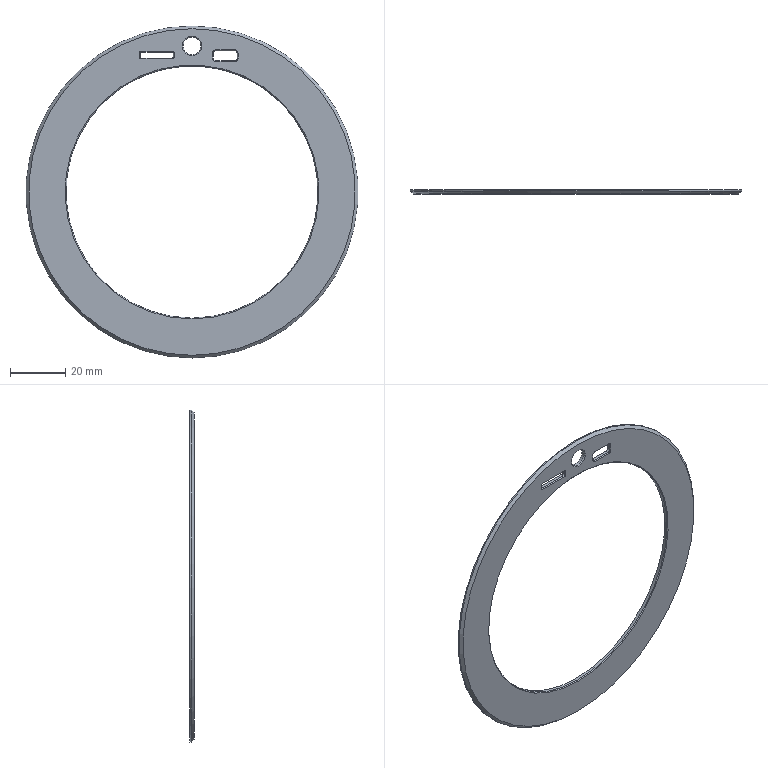Part | NX | 1 solid | 40 faces | box 119.8 x 1.45 x 119.8 mm | volume 6583 mm3 | plane 18 | cylinder 11 | cone 11 | commonest cylinder face diameters 0.6 x4 2 x4 6.4 x1 91 x1 119.8 x1
STEP:
#1=CARTESIAN_POINT('',(-7.04,-1.45,48.03));
#2=VERTEX_POINT('',#1);
#3=CARTESIAN_POINT('',(-18.44,-1.45,48.03));
#4=VERTEX_POINT('',#3);
#5=CARTESIAN_POINT('',(0.,-1.45,48.03));
#6=DIRECTION('',(-1.,0.,0.));
#7=VECTOR('',#6,1000.);
#8=LINE('',#5,#7);
#9=EDGE_CURVE('',#2,#4,#8,.T.);
#10=ORIENTED_EDGE('',*,*,#9,.T.);
#11=CARTESIAN_POINT('',(-19.04,-1.45,48.63));
#12=VERTEX_POINT('',#11);
#13=CARTESIAN_POINT('',(-18.44,-1.45,48.63));
#14=DIRECTION('',(0.,-1.,0.));
#15=DIRECTION('',(0.,0.,-1.));
#16=AXIS2_PLACEMENT_3D('',#13,#14,#15);
#17=CIRCLE('',#16,0.6);
#18=EDGE_CURVE('',#4,#12,#17,.F.);
#19=ORIENTED_EDGE('',*,*,#18,.T.);
#20=CARTESIAN_POINT('',(-19.04,-1.45,50.08));
#21=VERTEX_POINT('',#20);
#22=CARTESIAN_POINT('',(-19.04,-1.45,0.));
#23=DIRECTION('',(0.,0.,1.));
#24=VECTOR('',#23,1000.);
#25=LINE('',#22,#24);
#26=EDGE_CURVE('',#12,#21,#25,.T.);
#27=ORIENTED_EDGE('',*,*,#26,.T.);
#28=CARTESIAN_POINT('',(-18.44,-1.45,50.68));
#29=VERTEX_POINT('',#28);
#30=CARTESIAN_POINT('',(-18.44,-1.45,50.08));
#31=DIRECTION('',(0.,-1.,0.));
#32=DIRECTION('',(0.,0.,-1.));
#33=AXIS2_PLACEMENT_3D('',#30,#31,#32);
#34=CIRCLE('',#33,0.6);
#35=EDGE_CURVE('',#21,#29,#34,.F.);
#36=ORIENTED_EDGE('',*,*,#35,.T.);
#37=CARTESIAN_POINT('',(-7.04,-1.45,50.68));
#38=VERTEX_POINT('',#37);
#39=CARTESIAN_POINT('',(0.,-1.45,50.68));
#40=DIRECTION('',(1.,0.,0.));
#41=VECTOR('',#40,1000.);
#42=LINE('',#39,#41);
#43=EDGE_CURVE('',#29,#38,#42,.T.);
#44=ORIENTED_EDGE('',*,*,#43,.T.);
#45=CARTESIAN_POINT('',(-6.44,-1.45,50.08));
#46=VERTEX_POINT('',#45);
#47=CARTESIAN_POINT('',(-7.04,-1.45,50.08));
#48=DIRECTION('',(0.,-1.,0.));
#49=DIRECTION('',(0.,0.,-1.));
#50=AXIS2_PLACEMENT_3D('',#47,#48,#49);
#51=CIRCLE('',#50,0.6);
#52=EDGE_CURVE('',#38,#46,#51,.F.);
#53=ORIENTED_EDGE('',*,*,#52,.T.);
#54=CARTESIAN_POINT('',(-6.44,-1.45,48.63));
#55=VERTEX_POINT('',#54);
#56=CARTESIAN_POINT('',(-6.44,-1.45,0.));
#57=DIRECTION('',(0.,0.,-1.));
#58=VECTOR('',#57,1000.);
#59=LINE('',#56,#58);
#60=EDGE_CURVE('',#46,#55,#59,.T.);
#61=ORIENTED_EDGE('',*,*,#60,.T.);
#62=CARTESIAN_POINT('',(-7.04,-1.45,48.63));
#63=DIRECTION('',(0.,-1.,0.));
#64=DIRECTION('',(0.,0.,-1.));
#65=AXIS2_PLACEMENT_3D('',#62,#63,#64);
#66=CIRCLE('',#65,0.6);
#67=EDGE_CURVE('',#55,#2,#66,.F.);
#68=ORIENTED_EDGE('',*,*,#67,.T.);
#69=EDGE_LOOP('',(#10,#19,#27,#36,#44,#53,#61,#68));
#70=FACE_BOUND('',#69,.T.);
#71=CARTESIAN_POINT('',(0.,-1.45,49.2));
#72=VERTEX_POINT('',#71);
#73=CARTESIAN_POINT('',(0.,-1.45,52.7));
#74=DIRECTION('',(0.,-1.,0.));
#75=DIRECTION('',(0.,0.,-1.));
#76=AXIS2_PLACEMENT_3D('',#73,#74,#75);
#77=CIRCLE('',#76,3.5);
#78=EDGE_CURVE('',#72,#72,#77,.F.);
#79=ORIENTED_EDGE('',*,*,#78,.T.);
#80=EDGE_LOOP('',(#79));
#81=FACE_BOUND('',#80,.T.);
#82=CARTESIAN_POINT('',(15.33,-1.45,47.05));
#83=VERTEX_POINT('',#82);
#84=CARTESIAN_POINT('',(8.6,-1.45,47.05));
#85=VERTEX_POINT('',#84);
#86=CARTESIAN_POINT('',(0.,-1.45,47.05));
#87=DIRECTION('',(-1.,0.,0.));
#88=VECTOR('',#87,1000.);
#89=LINE('',#86,#88);
#90=EDGE_CURVE('',#83,#85,#89,.T.);
#91=ORIENTED_EDGE('',*,*,#90,.T.);
#92=CARTESIAN_POINT('',(7.3,-1.45,48.35));
#93=VERTEX_POINT('',#92);
#94=CARTESIAN_POINT('',(8.6,-1.45,48.35));
#95=DIRECTION('',(0.,-1.,0.));
#96=DIRECTION('',(0.,0.,-1.));
#97=AXIS2_PLACEMENT_3D('',#94,#95,#96);
#98=CIRCLE('',#97,1.3);
#99=EDGE_CURVE('',#85,#93,#98,.F.);
#100=ORIENTED_EDGE('',*,*,#99,.T.);
#101=CARTESIAN_POINT('',(7.3,-1.45,50.05));
#102=VERTEX_POINT('',#101);
#103=CARTESIAN_POINT('',(7.3,-1.45,0.));
#104=DIRECTION('',(0.,0.,1.));
#105=VECTOR('',#104,1000.);
#106=LINE('',#103,#105);
#107=EDGE_CURVE('',#93,#102,#106,.T.);
#108=ORIENTED_EDGE('',*,*,#107,.T.);
#109=CARTESIAN_POINT('',(8.6,-1.45,51.35));
#110=VERTEX_POINT('',#109);
#111=CARTESIAN_POINT('',(8.6,-1.45,50.05));
#112=DIRECTION('',(0.,-1.,0.));
#113=DIRECTION('',(0.,0.,-1.));
#114=AXIS2_PLACEMENT_3D('',#111,#112,#113);
#115=CIRCLE('',#114,1.3);
#116=EDGE_CURVE('',#102,#110,#115,.F.);
#117=ORIENTED_EDGE('',*,*,#116,.T.);
#118=CARTESIAN_POINT('',(15.33,-1.45,51.35));
#119=VERTEX_POINT('',#118);
#120=CARTESIAN_POINT('',(0.,-1.45,51.35));
#121=DIRECTION('',(1.,0.,0.));
#122=VECTOR('',#121,1000.);
#123=LINE('',#120,#122);
#124=EDGE_CURVE('',#110,#119,#123,.T.);
#125=ORIENTED_EDGE('',*,*,#124,.T.);
#126=CARTESIAN_POINT('',(16.63,-1.45,50.05));
#127=VERTEX_POINT('',#126);
#128=CARTESIAN_POINT('',(15.33,-1.45,50.05));
#129=DIRECTION('',(0.,-1.,0.));
#130=DIRECTION('',(0.,0.,-1.));
#131=AXIS2_PLACEMENT_3D('',#128,#129,#130);
#132=CIRCLE('',#131,1.3);
#133=EDGE_CURVE('',#119,#127,#132,.F.);
#134=ORIENTED_EDGE('',*,*,#133,.T.);
#135=CARTESIAN_POINT('',(16.63,-1.45,48.35));
#136=VERTEX_POINT('',#135);
#137=CARTESIAN_POINT('',(16.63,-1.45,0.));
#138=DIRECTION('',(0.,0.,-1.));
#139=VECTOR('',#138,1000.);
#140=LINE('',#137,#139);
#141=EDGE_CURVE('',#127,#136,#140,.T.);
#142=ORIENTED_EDGE('',*,*,#141,.T.);
#143=CARTESIAN_POINT('',(15.33,-1.45,48.35));
#144=DIRECTION('',(0.,-1.,0.));
#145=DIRECTION('',(0.,0.,-1.));
#146=AXIS2_PLACEMENT_3D('',#143,#144,#145);
#147=CIRCLE('',#146,1.3);
#148=EDGE_CURVE('',#136,#83,#147,.F.);
#149=ORIENTED_EDGE('',*,*,#148,.T.);
#150=EDGE_LOOP('',(#91,#100,#108,#117,#125,#134,#142,#149));
#151=FACE_BOUND('',#150,.T.);
#152=CARTESIAN_POINT('',(0.,-1.45,-45.8));
#153=VERTEX_POINT('',#152);
#154=CARTESIAN_POINT('',(0.,-1.45,0.));
#155=DIRECTION('',(0.,-1.,0.));
#156=DIRECTION('',(0.,0.,-1.));
#157=AXIS2_PLACEMENT_3D('',#154,#155,#156);
#158=CIRCLE('',#157,45.8);
#159=EDGE_CURVE('',#153,#153,#158,.F.);
#160=ORIENTED_EDGE('',*,*,#159,.T.);
#161=EDGE_LOOP('',(#160));
#162=FACE_BOUND('',#161,.T.);
#163=CARTESIAN_POINT('',(0.,-1.45,-58.9));
#164=VERTEX_POINT('',#163);
#165=CARTESIAN_POINT('',(0.,-1.45,0.));
#166=DIRECTION('',(0.,-1.,0.));
#167=DIRECTION('',(0.,0.,-1.));
#168=AXIS2_PLACEMENT_3D('',#165,#166,#167);
#169=CIRCLE('',#168,58.9);
#170=EDGE_CURVE('',#164,#164,#169,.T.);
#171=ORIENTED_EDGE('',*,*,#170,.T.);
#172=EDGE_LOOP('',(#171));
#173=FACE_BOUND('',#172,.T.);
#174=CARTESIAN_POINT('',(0.,-1.45,0.));
#175=DIRECTION('',(0.,-1.,0.));
#176=DIRECTION('',(0.,0.,1.));
#177=AXIS2_PLACEMENT_3D('',#174,#175,#176);
#178=PLANE('',#177);
#179=ADVANCED_FACE('',(#70,#81,#151,#162,#173),#178,.T.);
#180=CARTESIAN_POINT('',(15.33,0.,51.05));
#181=VERTEX_POINT('',#180);
#182=CARTESIAN_POINT('',(8.6,0.,51.05));
#183=VERTEX_POINT('',#182);
#184=CARTESIAN_POINT('',(16.33,0.,51.05));
#185=DIRECTION('',(-1.,0.,0.));
#186=VECTOR('',#185,1000.);
#187=LINE('',#184,#186);
#188=EDGE_CURVE('',#181,#183,#187,.T.);
#189=ORIENTED_EDGE('',*,*,#188,.T.);
#190=CARTESIAN_POINT('',(7.6,0.,50.05));
#191=VERTEX_POINT('',#190);
#192=CARTESIAN_POINT('',(8.6,0.,50.05));
#193=DIRECTION('',(0.,-1.,0.));
#194=DIRECTION('',(0.,0.,1.));
#195=AXIS2_PLACEMENT_3D('',#192,#193,#194);
#196=CIRCLE('',#195,1.);
#197=EDGE_CURVE('',#183,#191,#196,.T.);
#198=ORIENTED_EDGE('',*,*,#197,.T.);
#199=CARTESIAN_POINT('',(7.6,0.,48.35));
#200=VERTEX_POINT('',#199);
#201=CARTESIAN_POINT('',(7.6,0.,47.35));
#202=DIRECTION('',(0.,0.,-1.));
#203=VECTOR('',#202,1000.);
#204=LINE('',#201,#203);
#205=EDGE_CURVE('',#191,#200,#204,.T.);
#206=ORIENTED_EDGE('',*,*,#205,.T.);
#207=CARTESIAN_POINT('',(8.6,0.,47.35));
#208=VERTEX_POINT('',#207);
#209=CARTESIAN_POINT('',(8.6,0.,48.35));
#210=DIRECTION('',(0.,-1.,0.));
#211=DIRECTION('',(0.,0.,1.));
#212=AXIS2_PLACEMENT_3D('',#209,#210,#211);
#213=CIRCLE('',#212,1.);
#214=EDGE_CURVE('',#200,#208,#213,.T.);
#215=ORIENTED_EDGE('',*,*,#214,.T.);
#216=CARTESIAN_POINT('',(15.33,0.,47.35));
#217=VERTEX_POINT('',#216);
#218=CARTESIAN_POINT('',(16.33,0.,47.35));
#219=DIRECTION('',(1.,0.,0.));
#220=VECTOR('',#219,1000.);
#221=LINE('',#218,#220);
#222=EDGE_CURVE('',#208,#217,#221,.T.);
#223=ORIENTED_EDGE('',*,*,#222,.T.);
#224=CARTESIAN_POINT('',(16.33,0.,48.35));
#225=VERTEX_POINT('',#224);
#226=CARTESIAN_POINT('',(15.33,0.,48.35));
#227=DIRECTION('',(0.,-1.,0.));
#228=DIRECTION('',(0.,0.,1.));
#229=AXIS2_PLACEMENT_3D('',#226,#227,#228);
#230=CIRCLE('',#229,1.);
#231=EDGE_CURVE('',#217,#225,#230,.T.);
#232=ORIENTED_EDGE('',*,*,#231,.T.);
#233=CARTESIAN_POINT('',(16.33,0.,50.05));
#234=VERTEX_POINT('',#233);
#235=CARTESIAN_POINT('',(16.33,0.,47.35));
#236=DIRECTION('',(0.,0.,1.));
#237=VECTOR('',#236,1000.);
#238=LINE('',#235,#237);
#239=EDGE_CURVE('',#225,#234,#238,.T.);
#240=ORIENTED_EDGE('',*,*,#239,.T.);
#241=CARTESIAN_POINT('',(15.33,0.,50.05));
#242=DIRECTION('',(0.,-1.,0.));
#243=DIRECTION('',(0.,0.,1.));
#244=AXIS2_PLACEMENT_3D('',#241,#242,#243);
#245=CIRCLE('',#244,1.);
#246=EDGE_CURVE('',#234,#181,#245,.T.);
#247=ORIENTED_EDGE('',*,*,#246,.T.);
#248=EDGE_LOOP('',(#189,#198,#206,#215,#223,#232,#240,#247));
#249=FACE_BOUND('',#248,.T.);
#250=CARTESIAN_POINT('',(0.,0.,45.5));
#251=VERTEX_POINT('',#250);
#252=CARTESIAN_POINT('',(0.,0.,0.));
#253=DIRECTION('',(0.,-1.,0.));
#254=DIRECTION('',(0.,0.,1.));
#255=AXIS2_PLACEMENT_3D('',#252,#253,#254);
#256=CIRCLE('',#255,45.5);
#257=EDGE_CURVE('',#251,#251,#256,.T.);
#258=ORIENTED_EDGE('',*,*,#257,.T.);
#259=EDGE_LOOP('',(#258));
#260=FACE_BOUND('',#259,.T.);
#261=CARTESIAN_POINT('',(0.,0.,59.9));
#262=VERTEX_POINT('',#261);
#263=CARTESIAN_POINT('',(0.,0.,0.));
#264=DIRECTION('',(0.,-1.,0.));
#265=DIRECTION('',(0.,0.,1.));
#266=AXIS2_PLACEMENT_3D('',#263,#264,#265);
#267=CIRCLE('',#266,59.9);
#268=EDGE_CURVE('',#262,#262,#267,.T.);
#269=ORIENTED_EDGE('',*,*,#268,.F.);
#270=EDGE_LOOP('',(#269));
#271=FACE_BOUND('',#270,.T.);
#272=CARTESIAN_POINT('',(0.,0.,55.9));
#273=VERTEX_POINT('',#272);
#274=CARTESIAN_POINT('',(0.,0.,52.7));
#275=DIRECTION('',(0.,-1.,0.));
#276=DIRECTION('',(0.,0.,1.));
#277=AXIS2_PLACEMENT_3D('',#274,#275,#276);
#278=CIRCLE('',#277,3.2);
#279=EDGE_CURVE('',#273,#273,#278,.T.);
#280=ORIENTED_EDGE('',*,*,#279,.T.);
#281=EDGE_LOOP('',(#280));
#282=FACE_BOUND('',#281,.T.);
#283=CARTESIAN_POINT('',(-7.04,0.,50.38));
#284=VERTEX_POINT('',#283);
#285=CARTESIAN_POINT('',(-18.44,0.,50.38));
#286=VERTEX_POINT('',#285);
#287=CARTESIAN_POINT('',(-6.74,0.,50.38));
#288=DIRECTION('',(-1.,0.,0.));
#289=VECTOR('',#288,1000.);
#290=LINE('',#287,#289);
#291=EDGE_CURVE('',#284,#286,#290,.T.);
#292=ORIENTED_EDGE('',*,*,#291,.T.);
#293=CARTESIAN_POINT('',(-18.74,0.,50.08));
#294=VERTEX_POINT('',#293);
#295=CARTESIAN_POINT('',(-18.44,0.,50.08));
#296=DIRECTION('',(0.,-1.,0.));
#297=DIRECTION('',(0.,0.,1.));
#298=AXIS2_PLACEMENT_3D('',#295,#296,#297);
#299=CIRCLE('',#298,0.3);
#300=EDGE_CURVE('',#286,#294,#299,.T.);
#301=ORIENTED_EDGE('',*,*,#300,.T.);
#302=CARTESIAN_POINT('',(-18.74,0.,48.63));
#303=VERTEX_POINT('',#302);
#304=CARTESIAN_POINT('',(-18.74,0.,48.33));
#305=DIRECTION('',(0.,0.,-1.));
#306=VECTOR('',#305,1000.);
#307=LINE('',#304,#306);
#308=EDGE_CURVE('',#294,#303,#307,.T.);
#309=ORIENTED_EDGE('',*,*,#308,.T.);
#310=CARTESIAN_POINT('',(-18.44,0.,48.33));
#311=VERTEX_POINT('',#310);
#312=CARTESIAN_POINT('',(-18.44,0.,48.63));
#313=DIRECTION('',(0.,-1.,0.));
#314=DIRECTION('',(0.,0.,1.));
#315=AXIS2_PLACEMENT_3D('',#312,#313,#314);
#316=CIRCLE('',#315,0.3);
#317=EDGE_CURVE('',#303,#311,#316,.T.);
#318=ORIENTED_EDGE('',*,*,#317,.T.);
#319=CARTESIAN_POINT('',(-7.04,0.,48.33));
#320=VERTEX_POINT('',#319);
#321=CARTESIAN_POINT('',(-6.74,0.,48.33));
#322=DIRECTION('',(1.,0.,0.));
#323=VECTOR('',#322,1000.);
#324=LINE('',#321,#323);
#325=EDGE_CURVE('',#311,#320,#324,.T.);
#326=ORIENTED_EDGE('',*,*,#325,.T.);
#327=CARTESIAN_POINT('',(-6.74,0.,48.63));
#328=VERTEX_POINT('',#327);
#329=CARTESIAN_POINT('',(-7.04,0.,48.63));
#330=DIRECTION('',(0.,-1.,0.));
#331=DIRECTION('',(0.,0.,1.));
#332=AXIS2_PLACEMENT_3D('',#329,#330,#331);
#333=CIRCLE('',#332,0.3);
#334=EDGE_CURVE('',#320,#328,#333,.T.);
#335=ORIENTED_EDGE('',*,*,#334,.T.);
#336=CARTESIAN_POINT('',(-6.74,0.,50.08));
#337=VERTEX_POINT('',#336);
#338=CARTESIAN_POINT('',(-6.74,0.,48.33));
#339=DIRECTION('',(0.,0.,1.));
#340=VECTOR('',#339,1000.);
#341=LINE('',#338,#340);
#342=EDGE_CURVE('',#328,#337,#341,.T.);
#343=ORIENTED_EDGE('',*,*,#342,.T.);
#344=CARTESIAN_POINT('',(-7.04,0.,50.08));
#345=DIRECTION('',(0.,-1.,0.));
#346=DIRECTION('',(0.,0.,1.));
#347=AXIS2_PLACEMENT_3D('',#344,#345,#346);
#348=CIRCLE('',#347,0.3);
#349=EDGE_CURVE('',#337,#284,#348,.T.);
#350=ORIENTED_EDGE('',*,*,#349,.T.);
#351=EDGE_LOOP('',(#292,#301,#309,#318,#326,#335,#343,#350));
#352=FACE_BOUND('',#351,.T.);
#353=CARTESIAN_POINT('',(0.,0.,0.));
#354=DIRECTION('',(0.,-1.,0.));
#355=DIRECTION('',(0.,0.,1.));
#356=AXIS2_PLACEMENT_3D('',#353,#354,#355);
#357=PLANE('',#356);
#358=ADVANCED_FACE('',(#249,#260,#271,#282,#352),#357,.F.);
#359=CARTESIAN_POINT('',(0.,-0.45,-59.9));
#360=VERTEX_POINT('',#359);
#361=CARTESIAN_POINT('',(0.,-0.45,0.));
#362=DIRECTION('',(0.,-1.,0.));
#363=DIRECTION('',(0.,0.,-1.));
#364=AXIS2_PLACEMENT_3D('',#361,#362,#363);
#365=CIRCLE('',#364,59.9);
#366=EDGE_CURVE('',#360,#360,#365,.F.);
#367=ORIENTED_EDGE('',*,*,#366,.T.);
#368=EDGE_LOOP('',(#367));
#369=FACE_BOUND('',#368,.T.);
#370=ORIENTED_EDGE('',*,*,#268,.T.);
#371=EDGE_LOOP('',(#370));
#372=FACE_BOUND('',#371,.T.);
#373=CARTESIAN_POINT('',(0.,-1.45,0.));
#374=DIRECTION('',(0.,1.,0.));
#375=DIRECTION('',(0.,0.,-1.));
#376=AXIS2_PLACEMENT_3D('',#373,#374,#375);
#377=CYLINDRICAL_SURFACE('',#376,59.9);
#378=ADVANCED_FACE('',(#369,#372),#377,.T.);
#379=CARTESIAN_POINT('',(0.,-1.15,-45.5));
#380=VERTEX_POINT('',#379);
#381=CARTESIAN_POINT('',(0.,-1.15,0.));
#382=DIRECTION('',(0.,-1.,0.));
#383=DIRECTION('',(0.,0.,-1.));
#384=AXIS2_PLACEMENT_3D('',#381,#382,#383);
#385=CIRCLE('',#384,45.5);
#386=EDGE_CURVE('',#380,#380,#385,.T.);
#387=ORIENTED_EDGE('',*,*,#386,.T.);
#388=EDGE_LOOP('',(#387));
#389=FACE_BOUND('',#388,.T.);
#390=ORIENTED_EDGE('',*,*,#257,.F.);
#391=EDGE_LOOP('',(#390));
#392=FACE_BOUND('',#391,.T.);
#393=CARTESIAN_POINT('',(0.,-1.45,0.));
#394=DIRECTION('',(0.,1.,0.));
#395=DIRECTION('',(0.,0.,-1.));
#396=AXIS2_PLACEMENT_3D('',#393,#394,#395);
#397=CYLINDRICAL_SURFACE('',#396,45.5);
#398=ADVANCED_FACE('',(#389,#392),#397,.F.);
#399=CARTESIAN_POINT('',(0.,-1.15,49.5));
#400=VERTEX_POINT('',#399);
#401=CARTESIAN_POINT('',(0.,-1.15,52.7));
#402=DIRECTION('',(0.,-1.,0.));
#403=DIRECTION('',(0.,0.,-1.));
#404=AXIS2_PLACEMENT_3D('',#401,#402,#403);
#405=CIRCLE('',#404,3.2);
#406=EDGE_CURVE('',#400,#400,#405,.T.);
#407=ORIENTED_EDGE('',*,*,#406,.T.);
#408=EDGE_LOOP('',(#407));
#409=FACE_BOUND('',#408,.T.);
#410=ORIENTED_EDGE('',*,*,#279,.F.);
#411=EDGE_LOOP('',(#410));
#412=FACE_BOUND('',#411,.T.);
#413=CARTESIAN_POINT('',(0.,-1.45,52.7));
#414=DIRECTION('',(0.,1.,0.));
#415=DIRECTION('',(0.,0.,-1.));
#416=AXIS2_PLACEMENT_3D('',#413,#414,#415);
#417=CYLINDRICAL_SURFACE('',#416,3.2);
#418=ADVANCED_FACE('',(#409,#412),#417,.F.);
#419=CARTESIAN_POINT('',(7.6,-1.15,50.05));
#420=VERTEX_POINT('',#419);
#421=CARTESIAN_POINT('',(7.6,-1.45,50.05));
#422=DIRECTION('',(0.,1.,0.));
#423=VECTOR('',#422,1000.);
#424=LINE('',#421,#423);
#425=EDGE_CURVE('',#191,#420,#424,.F.);
#426=ORIENTED_EDGE('',*,*,#425,.T.);
#427=CARTESIAN_POINT('',(7.6,-1.15,48.35));
#428=VERTEX_POINT('',#427);
#429=CARTESIAN_POINT('',(7.6,-1.15,47.35));
#430=DIRECTION('',(0.,0.,-1.));
#431=VECTOR('',#430,1000.);
#432=LINE('',#429,#431);
#433=EDGE_CURVE('',#420,#428,#432,.T.);
#434=ORIENTED_EDGE('',*,*,#433,.T.);
#435=CARTESIAN_POINT('',(7.6,0.,48.35));
#436=DIRECTION('',(0.,1.,0.));
#437=VECTOR('',#436,1000.);
#438=LINE('',#435,#437);
#439=EDGE_CURVE('',#428,#200,#438,.T.);
#440=ORIENTED_EDGE('',*,*,#439,.T.);
#441=ORIENTED_EDGE('',*,*,#205,.F.);
#442=EDGE_LOOP('',(#426,#434,#440,#441));
#443=FACE_BOUND('',#442,.T.);
#444=CARTESIAN_POINT('',(7.6,-1.45,47.35));
#445=DIRECTION('',(1.,0.,0.));
#446=DIRECTION('',(0.,0.,1.));
#447=AXIS2_PLACEMENT_3D('',#444,#445,#446);
#448=PLANE('',#447);
#449=ADVANCED_FACE('',(#443),#448,.T.);
#450=CARTESIAN_POINT('',(8.6,-1.15,47.35));
#451=VERTEX_POINT('',#450);
#452=CARTESIAN_POINT('',(8.6,-1.45,47.35));
#453=DIRECTION('',(0.,1.,0.));
#454=VECTOR('',#453,1000.);
#455=LINE('',#452,#454);
#456=EDGE_CURVE('',#208,#451,#455,.F.);
#457=ORIENTED_EDGE('',*,*,#456,.T.);
#458=CARTESIAN_POINT('',(15.33,-1.15,47.35));
#459=VERTEX_POINT('',#458);
#460=CARTESIAN_POINT('',(16.33,-1.15,47.35));
#461=DIRECTION('',(1.,0.,0.));
#462=VECTOR('',#461,1000.);
#463=LINE('',#460,#462);
#464=EDGE_CURVE('',#451,#459,#463,.T.);
#465=ORIENTED_EDGE('',*,*,#464,.T.);
#466=CARTESIAN_POINT('',(15.33,0.,47.35));
#467=DIRECTION('',(0.,1.,0.));
#468=VECTOR('',#467,1000.);
#469=LINE('',#466,#468);
#470=EDGE_CURVE('',#459,#217,#469,.T.);
#471=ORIENTED_EDGE('',*,*,#470,.T.);
#472=ORIENTED_EDGE('',*,*,#222,.F.);
#473=EDGE_LOOP('',(#457,#465,#471,#472));
#474=FACE_BOUND('',#473,.T.);
#475=CARTESIAN_POINT('',(16.33,-1.45,47.35));
#476=DIRECTION('',(0.,0.,1.));
#477=DIRECTION('',(-1.,0.,0.));
#478=AXIS2_PLACEMENT_3D('',#475,#476,#477);
#479=PLANE('',#478);
#480=ADVANCED_FACE('',(#474),#479,.T.);
#481=CARTESIAN_POINT('',(16.33,-1.15,48.35));
#482=VERTEX_POINT('',#481);
#483=CARTESIAN_POINT('',(16.33,-1.45,48.35));
#484=DIRECTION('',(0.,1.,0.));
#485=VECTOR('',#484,1000.);
#486=LINE('',#483,#485);
#487=EDGE_CURVE('',#225,#482,#486,.F.);
#488=ORIENTED_EDGE('',*,*,#487,.T.);
#489=CARTESIAN_POINT('',(16.33,-1.15,50.05));
#490=VERTEX_POINT('',#489);
#491=CARTESIAN_POINT('',(16.33,-1.15,47.35));
#492=DIRECTION('',(0.,0.,1.));
#493=VECTOR('',#492,1000.);
#494=LINE('',#491,#493);
#495=EDGE_CURVE('',#482,#490,#494,.T.);
#496=ORIENTED_EDGE('',*,*,#495,.T.);
#497=CARTESIAN_POINT('',(16.33,0.,50.05));
#498=DIRECTION('',(0.,1.,0.));
#499=VECTOR('',#498,1000.);
#500=LINE('',#497,#499);
#501=EDGE_CURVE('',#490,#234,#500,.T.);
#502=ORIENTED_EDGE('',*,*,#501,.T.);
#503=ORIENTED_EDGE('',*,*,#239,.F.);
#504=EDGE_LOOP('',(#488,#496,#502,#503));
#505=FACE_BOUND('',#504,.T.);
#506=CARTESIAN_POINT('',(16.33,-1.45,47.35));
#507=DIRECTION('',(-1.,0.,0.));
#508=DIRECTION('',(0.,0.,-1.));
#509=AXIS2_PLACEMENT_3D('',#506,#507,#508);
#510=PLANE('',#509);
#511=ADVANCED_FACE('',(#505),#510,.T.);
#512=CARTESIAN_POINT('',(15.33,-1.15,51.05));
#513=VERTEX_POINT('',#512);
#514=CARTESIAN_POINT('',(15.33,-1.45,51.05));
#515=DIRECTION('',(0.,1.,0.));
#516=VECTOR('',#515,1000.);
#517=LINE('',#514,#516);
#518=EDGE_CURVE('',#181,#513,#517,.F.);
#519=ORIENTED_EDGE('',*,*,#518,.T.);
#520=CARTESIAN_POINT('',(8.6,-1.15,51.05));
#521=VERTEX_POINT('',#520);
#522=CARTESIAN_POINT('',(16.33,-1.15,51.05));
#523=DIRECTION('',(-1.,0.,0.));
#524=VECTOR('',#523,1000.);
#525=LINE('',#522,#524);
#526=EDGE_CURVE('',#513,#521,#525,.T.);
#527=ORIENTED_EDGE('',*,*,#526,.T.);
#528=CARTESIAN_POINT('',(8.6,0.,51.05));
#529=DIRECTION('',(0.,1.,0.));
#530=VECTOR('',#529,1000.);
#531=LINE('',#528,#530);
#532=EDGE_CURVE('',#521,#183,#531,.T.);
#533=ORIENTED_EDGE('',*,*,#532,.T.);
#534=ORIENTED_EDGE('',*,*,#188,.F.);
#535=EDGE_LOOP('',(#519,#527,#533,#534));
#536=FACE_BOUND('',#535,.T.);
#537=CARTESIAN_POINT('',(16.33,-1.45,51.05));
#538=DIRECTION('',(0.,0.,-1.));
#539=DIRECTION('',(1.,0.,0.));
#540=AXIS2_PLACEMENT_3D('',#537,#538,#539);
#541=PLANE('',#540);
#542=ADVANCED_FACE('',(#536),#541,.T.);
#543=CARTESIAN_POINT('',(-18.74,-1.15,50.08));
#544=VERTEX_POINT('',#543);
#545=CARTESIAN_POINT('',(-18.74,-1.45,50.08));
#546=DIRECTION('',(0.,1.,0.));
#547=VECTOR('',#546,1000.);
#548=LINE('',#545,#547);
#549=EDGE_CURVE('',#294,#544,#548,.F.);
#550=ORIENTED_EDGE('',*,*,#549,.T.);
#551=CARTESIAN_POINT('',(-18.74,-1.15,48.63));
#552=VERTEX_POINT('',#551);
#553=CARTESIAN_POINT('',(-18.74,-1.15,48.33));
#554=DIRECTION('',(0.,0.,-1.));
#555=VECTOR('',#554,1000.);
#556=LINE('',#553,#555);
#557=EDGE_CURVE('',#544,#552,#556,.T.);
#558=ORIENTED_EDGE('',*,*,#557,.T.);
#559=CARTESIAN_POINT('',(-18.74,0.,48.63));
#560=DIRECTION('',(0.,1.,0.));
#561=VECTOR('',#560,1000.);
#562=LINE('',#559,#561);
#563=EDGE_CURVE('',#552,#303,#562,.T.);
#564=ORIENTED_EDGE('',*,*,#563,.T.);
#565=ORIENTED_EDGE('',*,*,#308,.F.);
#566=EDGE_LOOP('',(#550,#558,#564,#565));
#567=FACE_BOUND('',#566,.T.);
#568=CARTESIAN_POINT('',(-18.74,-1.45,48.33));
#569=DIRECTION('',(1.,0.,0.));
#570=DIRECTION('',(0.,0.,1.));
#571=AXIS2_PLACEMENT_3D('',#568,#569,#570);
#572=PLANE('',#571);
#573=ADVANCED_FACE('',(#567),#572,.T.);
#574=CARTESIAN_POINT('',(-18.44,-1.15,48.33));
#575=VERTEX_POINT('',#574);
#576=CARTESIAN_POINT('',(-18.44,-1.45,48.33));
#577=DIRECTION('',(0.,1.,0.));
#578=VECTOR('',#577,1000.);
#579=LINE('',#576,#578);
#580=EDGE_CURVE('',#311,#575,#579,.F.);
#581=ORIENTED_EDGE('',*,*,#580,.T.);
#582=CARTESIAN_POINT('',(-7.04,-1.15,48.33));
#583=VERTEX_POINT('',#582);
#584=CARTESIAN_POINT('',(-6.74,-1.15,48.33));
#585=DIRECTION('',(1.,0.,0.));
#586=VECTOR('',#585,1000.);
#587=LINE('',#584,#586);
#588=EDGE_CURVE('',#575,#583,#587,.T.);
#589=ORIENTED_EDGE('',*,*,#588,.T.);
#590=CARTESIAN_POINT('',(-7.04,0.,48.33));
#591=DIRECTION('',(0.,1.,0.));
#592=VECTOR('',#591,1000.);
#593=LINE('',#590,#592);
#594=EDGE_CURVE('',#583,#320,#593,.T.);
#595=ORIENTED_EDGE('',*,*,#594,.T.);
#596=ORIENTED_EDGE('',*,*,#325,.F.);
#597=EDGE_LOOP('',(#581,#589,#595,#596));
#598=FACE_BOUND('',#597,.T.);
#599=CARTESIAN_POINT('',(-6.74,-1.45,48.33));
#600=DIRECTION('',(0.,0.,1.));
#601=DIRECTION('',(-1.,0.,0.));
#602=AXIS2_PLACEMENT_3D('',#599,#600,#601);
#603=PLANE('',#602);
#604=ADVANCED_FACE('',(#598),#603,.T.);
#605=CARTESIAN_POINT('',(-6.74,-1.15,48.63));
#606=VERTEX_POINT('',#605);
#607=CARTESIAN_POINT('',(-6.74,-1.45,48.63));
#608=DIRECTION('',(0.,1.,0.));
#609=VECTOR('',#608,1000.);
#610=LINE('',#607,#609);
#611=EDGE_CURVE('',#328,#606,#610,.F.);
#612=ORIENTED_EDGE('',*,*,#611,.T.);
#613=CARTESIAN_POINT('',(-6.74,-1.15,50.08));
#614=VERTEX_POINT('',#613);
#615=CARTESIAN_POINT('',(-6.74,-1.15,48.33));
#616=DIRECTION('',(0.,0.,1.));
#617=VECTOR('',#616,1000.);
#618=LINE('',#615,#617);
#619=EDGE_CURVE('',#606,#614,#618,.T.);
#620=ORIENTED_EDGE('',*,*,#619,.T.);
#621=CARTESIAN_POINT('',(-6.74,0.,50.08));
#622=DIRECTION('',(0.,1.,0.));
#623=VECTOR('',#622,1000.);
#624=LINE('',#621,#623);
#625=EDGE_CURVE('',#614,#337,#624,.T.);
#626=ORIENTED_EDGE('',*,*,#625,.T.);
#627=ORIENTED_EDGE('',*,*,#342,.F.);
#628=EDGE_LOOP('',(#612,#620,#626,#627));
#629=FACE_BOUND('',#628,.T.);
#630=CARTESIAN_POINT('',(-6.74,-1.45,48.33));
#631=DIRECTION('',(-1.,0.,0.));
#632=DIRECTION('',(0.,0.,-1.));
#633=AXIS2_PLACEMENT_3D('',#630,#631,#632);
#634=PLANE('',#633);
#635=ADVANCED_FACE('',(#629),#634,.T.);
#636=CARTESIAN_POINT('',(-7.04,-1.15,50.38));
#637=VERTEX_POINT('',#636);
#638=CARTESIAN_POINT('',(-7.04,-1.45,50.38));
#639=DIRECTION('',(0.,1.,0.));
#640=VECTOR('',#639,1000.);
#641=LINE('',#638,#640);
#642=EDGE_CURVE('',#284,#637,#641,.F.);
#643=ORIENTED_EDGE('',*,*,#642,.T.);
#644=CARTESIAN_POINT('',(-18.44,-1.15,50.38));
#645=VERTEX_POINT('',#644);
#646=CARTESIAN_POINT('',(-6.74,-1.15,50.38));
#647=DIRECTION('',(-1.,0.,0.));
#648=VECTOR('',#647,1000.);
#649=LINE('',#646,#648);
#650=EDGE_CURVE('',#637,#645,#649,.T.);
#651=ORIENTED_EDGE('',*,*,#650,.T.);
#652=CARTESIAN_POINT('',(-18.44,0.,50.38));
#653=DIRECTION('',(0.,1.,0.));
#654=VECTOR('',#653,1000.);
#655=LINE('',#652,#654);
#656=EDGE_CURVE('',#645,#286,#655,.T.);
#657=ORIENTED_EDGE('',*,*,#656,.T.);
#658=ORIENTED_EDGE('',*,*,#291,.F.);
#659=EDGE_LOOP('',(#643,#651,#657,#658));
#660=FACE_BOUND('',#659,.T.);
#661=CARTESIAN_POINT('',(-6.74,-1.45,50.38));
#662=DIRECTION('',(0.,0.,-1.));
#663=DIRECTION('',(1.,0.,0.));
#664=AXIS2_PLACEMENT_3D('',#661,#662,#663);
#665=PLANE('',#664);
#666=ADVANCED_FACE('',(#660),#665,.T.);
#667=ORIENTED_EDGE('',*,*,#532,.F.);
#668=CARTESIAN_POINT('',(8.6,-1.15,50.05));
#669=DIRECTION('',(0.,-1.,0.));
#670=DIRECTION('',(0.,0.,-1.));
#671=AXIS2_PLACEMENT_3D('',#668,#669,#670);
#672=CIRCLE('',#671,1.);
#673=EDGE_CURVE('',#521,#420,#672,.T.);
#674=ORIENTED_EDGE('',*,*,#673,.T.);
#675=ORIENTED_EDGE('',*,*,#425,.F.);
#676=ORIENTED_EDGE('',*,*,#197,.F.);
#677=EDGE_LOOP('',(#667,#674,#675,#676));
#678=FACE_BOUND('',#677,.T.);
#679=CARTESIAN_POINT('',(8.6,-1.45,50.05));
#680=DIRECTION('',(0.,-1.,0.));
#681=DIRECTION('',(0.,0.,1.));
#682=AXIS2_PLACEMENT_3D('',#679,#680,#681);
#683=CYLINDRICAL_SURFACE('',#682,1.);
#684=ADVANCED_FACE('',(#678),#683,.F.);
#685=ORIENTED_EDGE('',*,*,#439,.F.);
#686=CARTESIAN_POINT('',(8.6,-1.15,48.35));
#687=DIRECTION('',(0.,-1.,0.));
#688=DIRECTION('',(0.,0.,-1.));
#689=AXIS2_PLACEMENT_3D('',#686,#687,#688);
#690=CIRCLE('',#689,1.);
#691=EDGE_CURVE('',#428,#451,#690,.T.);
#692=ORIENTED_EDGE('',*,*,#691,.T.);
#693=ORIENTED_EDGE('',*,*,#456,.F.);
#694=ORIENTED_EDGE('',*,*,#214,.F.);
#695=EDGE_LOOP('',(#685,#692,#693,#694));
#696=FACE_BOUND('',#695,.T.);
#697=CARTESIAN_POINT('',(8.6,-1.45,48.35));
#698=DIRECTION('',(0.,-1.,0.));
#699=DIRECTION('',(0.,0.,1.));
#700=AXIS2_PLACEMENT_3D('',#697,#698,#699);
#701=CYLINDRICAL_SURFACE('',#700,1.);
#702=ADVANCED_FACE('',(#696),#701,.F.);
#703=ORIENTED_EDGE('',*,*,#501,.F.);
#704=CARTESIAN_POINT('',(15.33,-1.15,50.05));
#705=DIRECTION('',(0.,-1.,0.));
#706=DIRECTION('',(0.,0.,-1.));
#707=AXIS2_PLACEMENT_3D('',#704,#705,#706);
#708=CIRCLE('',#707,1.);
#709=EDGE_CURVE('',#490,#513,#708,.T.);
#710=ORIENTED_EDGE('',*,*,#709,.T.);
#711=ORIENTED_EDGE('',*,*,#518,.F.);
#712=ORIENTED_EDGE('',*,*,#246,.F.);
#713=EDGE_LOOP('',(#703,#710,#711,#712));
#714=FACE_BOUND('',#713,.T.);
#715=CARTESIAN_POINT('',(15.33,-1.45,50.05));
#716=DIRECTION('',(0.,-1.,0.));
#717=DIRECTION('',(0.,0.,1.));
#718=AXIS2_PLACEMENT_3D('',#715,#716,#717);
#719=CYLINDRICAL_SURFACE('',#718,1.);
#720=ADVANCED_FACE('',(#714),#719,.F.);
#721=ORIENTED_EDGE('',*,*,#470,.F.);
#722=CARTESIAN_POINT('',(15.33,-1.15,48.35));
#723=DIRECTION('',(0.,-1.,0.));
#724=DIRECTION('',(0.,0.,-1.));
#725=AXIS2_PLACEMENT_3D('',#722,#723,#724);
#726=CIRCLE('',#725,1.);
#727=EDGE_CURVE('',#459,#482,#726,.T.);
#728=ORIENTED_EDGE('',*,*,#727,.T.);
#729=ORIENTED_EDGE('',*,*,#487,.F.);
#730=ORIENTED_EDGE('',*,*,#231,.F.);
#731=EDGE_LOOP('',(#721,#728,#729,#730));
#732=FACE_BOUND('',#731,.T.);
#733=CARTESIAN_POINT('',(15.33,-1.45,48.35));
#734=DIRECTION('',(0.,-1.,0.));
#735=DIRECTION('',(0.,0.,1.));
#736=AXIS2_PLACEMENT_3D('',#733,#734,#735);
#737=CYLINDRICAL_SURFACE('',#736,1.);
#738=ADVANCED_FACE('',(#732),#737,.F.);
#739=ORIENTED_EDGE('',*,*,#656,.F.);
#740=CARTESIAN_POINT('',(-18.44,-1.15,50.08));
#741=DIRECTION('',(0.,-1.,0.));
#742=DIRECTION('',(0.,0.,-1.));
#743=AXIS2_PLACEMENT_3D('',#740,#741,#742);
#744=CIRCLE('',#743,0.3);
#745=EDGE_CURVE('',#645,#544,#744,.T.);
#746=ORIENTED_EDGE('',*,*,#745,.T.);
#747=ORIENTED_EDGE('',*,*,#549,.F.);
#748=ORIENTED_EDGE('',*,*,#300,.F.);
#749=EDGE_LOOP('',(#739,#746,#747,#748));
#750=FACE_BOUND('',#749,.T.);
#751=CARTESIAN_POINT('',(-18.44,-1.45,50.08));
#752=DIRECTION('',(0.,-1.,0.));
#753=DIRECTION('',(0.,0.,1.));
#754=AXIS2_PLACEMENT_3D('',#751,#752,#753);
#755=CYLINDRICAL_SURFACE('',#754,0.3);
#756=ADVANCED_FACE('',(#750),#755,.F.);
#757=ORIENTED_EDGE('',*,*,#563,.F.);
#758=CARTESIAN_POINT('',(-18.44,-1.15,48.63));
#759=DIRECTION('',(0.,-1.,0.));
#760=DIRECTION('',(0.,0.,-1.));
#761=AXIS2_PLACEMENT_3D('',#758,#759,#760);
#762=CIRCLE('',#761,0.3);
#763=EDGE_CURVE('',#552,#575,#762,.T.);
#764=ORIENTED_EDGE('',*,*,#763,.T.);
#765=ORIENTED_EDGE('',*,*,#580,.F.);
#766=ORIENTED_EDGE('',*,*,#317,.F.);
#767=EDGE_LOOP('',(#757,#764,#765,#766));
#768=FACE_BOUND('',#767,.T.);
#769=CARTESIAN_POINT('',(-18.44,-1.45,48.63));
#770=DIRECTION('',(0.,-1.,0.));
#771=DIRECTION('',(0.,0.,1.));
#772=AXIS2_PLACEMENT_3D('',#769,#770,#771);
#773=CYLINDRICAL_SURFACE('',#772,0.3);
#774=ADVANCED_FACE('',(#768),#773,.F.);
#775=ORIENTED_EDGE('',*,*,#625,.F.);
#776=CARTESIAN_POINT('',(-7.04,-1.15,50.08));
#777=DIRECTION('',(0.,-1.,0.));
#778=DIRECTION('',(0.,0.,-1.));
#779=AXIS2_PLACEMENT_3D('',#776,#777,#778);
#780=CIRCLE('',#779,0.3);
#781=EDGE_CURVE('',#614,#637,#780,.T.);
#782=ORIENTED_EDGE('',*,*,#781,.T.);
#783=ORIENTED_EDGE('',*,*,#642,.F.);
#784=ORIENTED_EDGE('',*,*,#349,.F.);
#785=EDGE_LOOP('',(#775,#782,#783,#784));
#786=FACE_BOUND('',#785,.T.);
#787=CARTESIAN_POINT('',(-7.04,-1.45,50.08));
#788=DIRECTION('',(0.,-1.,0.));
#789=DIRECTION('',(0.,0.,1.));
#790=AXIS2_PLACEMENT_3D('',#787,#788,#789);
#791=CYLINDRICAL_SURFACE('',#790,0.3);
#792=ADVANCED_FACE('',(#786),#791,.F.);
#793=ORIENTED_EDGE('',*,*,#594,.F.);
#794=CARTESIAN_POINT('',(-7.04,-1.15,48.63));
#795=DIRECTION('',(0.,-1.,0.));
#796=DIRECTION('',(0.,0.,-1.));
#797=AXIS2_PLACEMENT_3D('',#794,#795,#796);
#798=CIRCLE('',#797,0.3);
#799=EDGE_CURVE('',#583,#606,#798,.T.);
#800=ORIENTED_EDGE('',*,*,#799,.T.);
#801=ORIENTED_EDGE('',*,*,#611,.F.);
#802=ORIENTED_EDGE('',*,*,#334,.F.);
#803=EDGE_LOOP('',(#793,#800,#801,#802));
#804=FACE_BOUND('',#803,.T.);
#805=CARTESIAN_POINT('',(-7.04,-1.45,48.63));
#806=DIRECTION('',(0.,-1.,0.));
#807=DIRECTION('',(0.,0.,1.));
#808=AXIS2_PLACEMENT_3D('',#805,#806,#807);
#809=CYLINDRICAL_SURFACE('',#808,0.3);
#810=ADVANCED_FACE('',(#804),#809,.F.);
#811=ORIENTED_EDGE('',*,*,#366,.F.);
#812=EDGE_LOOP('',(#811));
#813=FACE_BOUND('',#812,.T.);
#814=ORIENTED_EDGE('',*,*,#170,.F.);
#815=EDGE_LOOP('',(#814));
#816=FACE_BOUND('',#815,.T.);
#817=CARTESIAN_POINT('',(0.,-1.45,0.));
#818=DIRECTION('',(0.,1.,0.));
#819=DIRECTION('',(0.,0.,1.));
#820=AXIS2_PLACEMENT_3D('',#817,#818,#819);
#821=CONICAL_SURFACE('',#820,58.9,0.7854);
#822=ADVANCED_FACE('',(#813,#816),#821,.T.);
#823=ORIENTED_EDGE('',*,*,#159,.F.);
#824=EDGE_LOOP('',(#823));
#825=FACE_BOUND('',#824,.T.);
#826=ORIENTED_EDGE('',*,*,#386,.F.);
#827=EDGE_LOOP('',(#826));
#828=FACE_BOUND('',#827,.T.);
#829=CARTESIAN_POINT('',(0.,-1.15,0.));
#830=DIRECTION('',(0.,-1.,0.));
#831=DIRECTION('',(0.,0.,-1.));
#832=AXIS2_PLACEMENT_3D('',#829,#830,#831);
#833=CONICAL_SURFACE('',#832,45.5,0.7854);
#834=ADVANCED_FACE('',(#825,#828),#833,.F.);
#835=CARTESIAN_POINT('',(-7.04,-1.15,50.38));
#836=DIRECTION('',(0.,-0.7071,0.7071));
#837=VECTOR('',#836,1000.);
#838=LINE('',#835,#837);
#839=EDGE_CURVE('',#637,#38,#838,.T.);
#840=ORIENTED_EDGE('',*,*,#839,.F.);
#841=ORIENTED_EDGE('',*,*,#781,.F.);
#842=CARTESIAN_POINT('',(-6.44,-1.45,50.08));
#843=DIRECTION('',(-0.7071,0.7071,0.));
#844=VECTOR('',#843,1000.);
#845=LINE('',#842,#844);
#846=EDGE_CURVE('',#46,#614,#845,.T.);
#847=ORIENTED_EDGE('',*,*,#846,.F.);
#848=ORIENTED_EDGE('',*,*,#52,.F.);
#849=EDGE_LOOP('',(#840,#841,#847,#848));
#850=FACE_BOUND('',#849,.T.);
#851=CARTESIAN_POINT('',(-7.04,-1.45,50.08));
#852=DIRECTION('',(0.,-1.,0.));
#853=DIRECTION('',(0.,0.,-1.));
#854=AXIS2_PLACEMENT_3D('',#851,#852,#853);
#855=CONICAL_SURFACE('',#854,0.6,0.7854);
#856=ADVANCED_FACE('',(#850),#855,.F.);
#857=ORIENTED_EDGE('',*,*,#846,.T.);
#858=ORIENTED_EDGE('',*,*,#619,.F.);
#859=CARTESIAN_POINT('',(-6.44,-1.45,48.63));
#860=DIRECTION('',(-0.7071,0.7071,0.));
#861=VECTOR('',#860,1000.);
#862=LINE('',#859,#861);
#863=EDGE_CURVE('',#55,#606,#862,.T.);
#864=ORIENTED_EDGE('',*,*,#863,.F.);
#865=ORIENTED_EDGE('',*,*,#60,.F.);
#866=EDGE_LOOP('',(#857,#858,#864,#865));
#867=FACE_BOUND('',#866,.T.);
#868=CARTESIAN_POINT('',(-6.74,-1.15,48.33));
#869=DIRECTION('',(0.7071,0.7071,0.));
#870=DIRECTION('',(0.,0.,1.));
#871=AXIS2_PLACEMENT_3D('',#868,#869,#870);
#872=PLANE('',#871);
#873=ADVANCED_FACE('',(#867),#872,.F.);
#874=ORIENTED_EDGE('',*,*,#839,.T.);
#875=ORIENTED_EDGE('',*,*,#43,.F.);
#876=CARTESIAN_POINT('',(-18.44,-1.15,50.38));
#877=DIRECTION('',(0.,-0.7071,0.7071));
#878=VECTOR('',#877,1000.);
#879=LINE('',#876,#878);
#880=EDGE_CURVE('',#645,#29,#879,.T.);
#881=ORIENTED_EDGE('',*,*,#880,.F.);
#882=ORIENTED_EDGE('',*,*,#650,.F.);
#883=EDGE_LOOP('',(#874,#875,#881,#882));
#884=FACE_BOUND('',#883,.T.);
#885=CARTESIAN_POINT('',(-6.74,-1.15,50.38));
#886=DIRECTION('',(0.,0.7071,0.7071));
#887=DIRECTION('',(-1.,0.,0.));
#888=AXIS2_PLACEMENT_3D('',#885,#886,#887);
#889=PLANE('',#888);
#890=ADVANCED_FACE('',(#884),#889,.F.);
#891=ORIENTED_EDGE('',*,*,#863,.T.);
#892=ORIENTED_EDGE('',*,*,#799,.F.);
#893=CARTESIAN_POINT('',(-7.04,-1.45,48.03));
#894=DIRECTION('',(0.,0.7071,0.7071));
#895=VECTOR('',#894,1000.);
#896=LINE('',#893,#895);
#897=EDGE_CURVE('',#2,#583,#896,.T.);
#898=ORIENTED_EDGE('',*,*,#897,.F.);
#899=ORIENTED_EDGE('',*,*,#67,.F.);
#900=EDGE_LOOP('',(#891,#892,#898,#899));
#901=FACE_BOUND('',#900,.T.);
#902=CARTESIAN_POINT('',(-7.04,-1.45,48.63));
#903=DIRECTION('',(0.,-1.,0.));
#904=DIRECTION('',(0.,0.,-1.));
#905=AXIS2_PLACEMENT_3D('',#902,#903,#904);
#906=CONICAL_SURFACE('',#905,0.6,0.7854);
#907=ADVANCED_FACE('',(#901),#906,.F.);
#908=ORIENTED_EDGE('',*,*,#880,.T.);
#909=ORIENTED_EDGE('',*,*,#35,.F.);
#910=CARTESIAN_POINT('',(-18.74,-1.15,50.08));
#911=DIRECTION('',(-0.7071,-0.7071,0.));
#912=VECTOR('',#911,1000.);
#913=LINE('',#910,#912);
#914=EDGE_CURVE('',#544,#21,#913,.T.);
#915=ORIENTED_EDGE('',*,*,#914,.F.);
#916=ORIENTED_EDGE('',*,*,#745,.F.);
#917=EDGE_LOOP('',(#908,#909,#915,#916));
#918=FACE_BOUND('',#917,.T.);
#919=CARTESIAN_POINT('',(-18.44,-1.45,50.08));
#920=DIRECTION('',(0.,-1.,0.));
#921=DIRECTION('',(0.,0.,-1.));
#922=AXIS2_PLACEMENT_3D('',#919,#920,#921);
#923=CONICAL_SURFACE('',#922,0.6,0.7854);
#924=ADVANCED_FACE('',(#918),#923,.F.);
#925=ORIENTED_EDGE('',*,*,#897,.T.);
#926=ORIENTED_EDGE('',*,*,#588,.F.);
#927=CARTESIAN_POINT('',(-18.44,-1.45,48.03));
#928=DIRECTION('',(0.,0.7071,0.7071));
#929=VECTOR('',#928,1000.);
#930=LINE('',#927,#929);
#931=EDGE_CURVE('',#4,#575,#930,.T.);
#932=ORIENTED_EDGE('',*,*,#931,.F.);
#933=ORIENTED_EDGE('',*,*,#9,.F.);
#934=EDGE_LOOP('',(#925,#926,#932,#933));
#935=FACE_BOUND('',#934,.T.);
#936=CARTESIAN_POINT('',(-6.74,-1.15,48.33));
#937=DIRECTION('',(0.,0.7071,-0.7071));
#938=DIRECTION('',(1.,0.,0.));
#939=AXIS2_PLACEMENT_3D('',#936,#937,#938);
#940=PLANE('',#939);
#941=ADVANCED_FACE('',(#935),#940,.F.);
#942=ORIENTED_EDGE('',*,*,#914,.T.);
#943=ORIENTED_EDGE('',*,*,#26,.F.);
#944=CARTESIAN_POINT('',(-18.74,-1.15,48.63));
#945=DIRECTION('',(-0.7071,-0.7071,0.));
#946=VECTOR('',#945,1000.);
#947=LINE('',#944,#946);
#948=EDGE_CURVE('',#552,#12,#947,.T.);
#949=ORIENTED_EDGE('',*,*,#948,.F.);
#950=ORIENTED_EDGE('',*,*,#557,.F.);
#951=EDGE_LOOP('',(#942,#943,#949,#950));
#952=FACE_BOUND('',#951,.T.);
#953=CARTESIAN_POINT('',(-18.74,-1.15,48.33));
#954=DIRECTION('',(-0.7071,0.7071,0.));
#955=DIRECTION('',(0.,0.,-1.));
#956=AXIS2_PLACEMENT_3D('',#953,#954,#955);
#957=PLANE('',#956);
#958=ADVANCED_FACE('',(#952),#957,.F.);
#959=ORIENTED_EDGE('',*,*,#931,.T.);
#960=ORIENTED_EDGE('',*,*,#763,.F.);
#961=ORIENTED_EDGE('',*,*,#948,.T.);
#962=ORIENTED_EDGE('',*,*,#18,.F.);
#963=EDGE_LOOP('',(#959,#960,#961,#962));
#964=FACE_BOUND('',#963,.T.);
#965=CARTESIAN_POINT('',(-18.44,-1.45,48.63));
#966=DIRECTION('',(0.,-1.,0.));
#967=DIRECTION('',(0.,0.,-1.));
#968=AXIS2_PLACEMENT_3D('',#965,#966,#967);
#969=CONICAL_SURFACE('',#968,0.6,0.7854);
#970=ADVANCED_FACE('',(#964),#969,.F.);
#971=ORIENTED_EDGE('',*,*,#78,.F.);
#972=EDGE_LOOP('',(#971));
#973=FACE_BOUND('',#972,.T.);
#974=ORIENTED_EDGE('',*,*,#406,.F.);
#975=EDGE_LOOP('',(#974));
#976=FACE_BOUND('',#975,.T.);
#977=CARTESIAN_POINT('',(0.,-1.15,52.7));
#978=DIRECTION('',(0.,-1.,0.));
#979=DIRECTION('',(0.,0.,-1.));
#980=AXIS2_PLACEMENT_3D('',#977,#978,#979);
#981=CONICAL_SURFACE('',#980,3.2,0.7854);
#982=ADVANCED_FACE('',(#973,#976),#981,.F.);
#983=CARTESIAN_POINT('',(15.33,-1.15,51.05));
#984=DIRECTION('',(0.,-0.7071,0.7071));
#985=VECTOR('',#984,1000.);
#986=LINE('',#983,#985);
#987=EDGE_CURVE('',#513,#119,#986,.T.);
#988=ORIENTED_EDGE('',*,*,#987,.F.);
#989=ORIENTED_EDGE('',*,*,#709,.F.);
#990=CARTESIAN_POINT('',(16.63,-1.45,50.05));
#991=DIRECTION('',(-0.7071,0.7071,0.));
#992=VECTOR('',#991,1000.);
#993=LINE('',#990,#992);
#994=EDGE_CURVE('',#127,#490,#993,.T.);
#995=ORIENTED_EDGE('',*,*,#994,.F.);
#996=ORIENTED_EDGE('',*,*,#133,.F.);
#997=EDGE_LOOP('',(#988,#989,#995,#996));
#998=FACE_BOUND('',#997,.T.);
#999=CARTESIAN_POINT('',(15.33,-1.45,50.05));
#1000=DIRECTION('',(0.,-1.,0.));
#1001=DIRECTION('',(0.,0.,-1.));
#1002=AXIS2_PLACEMENT_3D('',#999,#1000,#1001);
#1003=CONICAL_SURFACE('',#1002,1.3,0.7854);
#1004=ADVANCED_FACE('',(#998),#1003,.F.);
#1005=ORIENTED_EDGE('',*,*,#994,.T.);
#1006=ORIENTED_EDGE('',*,*,#495,.F.);
#1007=CARTESIAN_POINT('',(16.63,-1.45,48.35));
#1008=DIRECTION('',(-0.7071,0.7071,0.));
#1009=VECTOR('',#1008,1000.);
#1010=LINE('',#1007,#1009);
#1011=EDGE_CURVE('',#136,#482,#1010,.T.);
#1012=ORIENTED_EDGE('',*,*,#1011,.F.);
#1013=ORIENTED_EDGE('',*,*,#141,.F.);
#1014=EDGE_LOOP('',(#1005,#1006,#1012,#1013));
#1015=FACE_BOUND('',#1014,.T.);
#1016=CARTESIAN_POINT('',(16.33,-1.15,47.35));
#1017=DIRECTION('',(0.7071,0.7071,0.));
#1018=DIRECTION('',(0.,0.,1.));
#1019=AXIS2_PLACEMENT_3D('',#1016,#1017,#1018);
#1020=PLANE('',#1019);
#1021=ADVANCED_FACE('',(#1015),#1020,.F.);
#1022=ORIENTED_EDGE('',*,*,#987,.T.);
#1023=ORIENTED_EDGE('',*,*,#124,.F.);
#1024=CARTESIAN_POINT('',(8.6,-1.15,51.05));
#1025=DIRECTION('',(0.,-0.7071,0.7071));
#1026=VECTOR('',#1025,1000.);
#1027=LINE('',#1024,#1026);
#1028=EDGE_CURVE('',#521,#110,#1027,.T.);
#1029=ORIENTED_EDGE('',*,*,#1028,.F.);
#1030=ORIENTED_EDGE('',*,*,#526,.F.);
#1031=EDGE_LOOP('',(#1022,#1023,#1029,#1030));
#1032=FACE_BOUND('',#1031,.T.);
#1033=CARTESIAN_POINT('',(16.33,-1.15,51.05));
#1034=DIRECTION('',(0.,0.7071,0.7071));
#1035=DIRECTION('',(-1.,0.,0.));
#1036=AXIS2_PLACEMENT_3D('',#1033,#1034,#1035);
#1037=PLANE('',#1036);
#1038=ADVANCED_FACE('',(#1032),#1037,.F.);
#1039=ORIENTED_EDGE('',*,*,#1011,.T.);
#1040=ORIENTED_EDGE('',*,*,#727,.F.);
#1041=CARTESIAN_POINT('',(15.33,-1.45,47.05));
#1042=DIRECTION('',(0.,0.7071,0.7071));
#1043=VECTOR('',#1042,1000.);
#1044=LINE('',#1041,#1043);
#1045=EDGE_CURVE('',#83,#459,#1044,.T.);
#1046=ORIENTED_EDGE('',*,*,#1045,.F.);
#1047=ORIENTED_EDGE('',*,*,#148,.F.);
#1048=EDGE_LOOP('',(#1039,#1040,#1046,#1047));
#1049=FACE_BOUND('',#1048,.T.);
#1050=CARTESIAN_POINT('',(15.33,-1.45,48.35));
#1051=DIRECTION('',(0.,-1.,0.));
#1052=DIRECTION('',(0.,0.,-1.));
#1053=AXIS2_PLACEMENT_3D('',#1050,#1051,#1052);
#1054=CONICAL_SURFACE('',#1053,1.3,0.7854);
#1055=ADVANCED_FACE('',(#1049),#1054,.F.);
#1056=ORIENTED_EDGE('',*,*,#1028,.T.);
#1057=ORIENTED_EDGE('',*,*,#116,.F.);
#1058=CARTESIAN_POINT('',(7.6,-1.15,50.05));
#1059=DIRECTION('',(-0.7071,-0.7071,0.));
#1060=VECTOR('',#1059,1000.);
#1061=LINE('',#1058,#1060);
#1062=EDGE_CURVE('',#420,#102,#1061,.T.);
#1063=ORIENTED_EDGE('',*,*,#1062,.F.);
#1064=ORIENTED_EDGE('',*,*,#673,.F.);
#1065=EDGE_LOOP('',(#1056,#1057,#1063,#1064));
#1066=FACE_BOUND('',#1065,.T.);
#1067=CARTESIAN_POINT('',(8.6,-1.45,50.05));
#1068=DIRECTION('',(0.,-1.,0.));
#1069=DIRECTION('',(0.,0.,-1.));
#1070=AXIS2_PLACEMENT_3D('',#1067,#1068,#1069);
#1071=CONICAL_SURFACE('',#1070,1.3,0.7854);
#1072=ADVANCED_FACE('',(#1066),#1071,.F.);
#1073=ORIENTED_EDGE('',*,*,#1045,.T.);
#1074=ORIENTED_EDGE('',*,*,#464,.F.);
#1075=CARTESIAN_POINT('',(8.6,-1.45,47.05));
#1076=DIRECTION('',(0.,0.7071,0.7071));
#1077=VECTOR('',#1076,1000.);
#1078=LINE('',#1075,#1077);
#1079=EDGE_CURVE('',#85,#451,#1078,.T.);
#1080=ORIENTED_EDGE('',*,*,#1079,.F.);
#1081=ORIENTED_EDGE('',*,*,#90,.F.);
#1082=EDGE_LOOP('',(#1073,#1074,#1080,#1081));
#1083=FACE_BOUND('',#1082,.T.);
#1084=CARTESIAN_POINT('',(16.33,-1.15,47.35));
#1085=DIRECTION('',(0.,0.7071,-0.7071));
#1086=DIRECTION('',(1.,0.,0.));
#1087=AXIS2_PLACEMENT_3D('',#1084,#1085,#1086);
#1088=PLANE('',#1087);
#1089=ADVANCED_FACE('',(#1083),#1088,.F.);
#1090=ORIENTED_EDGE('',*,*,#1062,.T.);
#1091=ORIENTED_EDGE('',*,*,#107,.F.);
#1092=CARTESIAN_POINT('',(7.6,-1.15,48.35));
#1093=DIRECTION('',(-0.7071,-0.7071,0.));
#1094=VECTOR('',#1093,1000.);
#1095=LINE('',#1092,#1094);
#1096=EDGE_CURVE('',#428,#93,#1095,.T.);
#1097=ORIENTED_EDGE('',*,*,#1096,.F.);
#1098=ORIENTED_EDGE('',*,*,#433,.F.);
#1099=EDGE_LOOP('',(#1090,#1091,#1097,#1098));
#1100=FACE_BOUND('',#1099,.T.);
#1101=CARTESIAN_POINT('',(7.6,-1.15,47.35));
#1102=DIRECTION('',(-0.7071,0.7071,0.));
#1103=DIRECTION('',(0.,0.,-1.));
#1104=AXIS2_PLACEMENT_3D('',#1101,#1102,#1103);
#1105=PLANE('',#1104);
#1106=ADVANCED_FACE('',(#1100),#1105,.F.);
#1107=ORIENTED_EDGE('',*,*,#1079,.T.);
#1108=ORIENTED_EDGE('',*,*,#691,.F.);
#1109=ORIENTED_EDGE('',*,*,#1096,.T.);
#1110=ORIENTED_EDGE('',*,*,#99,.F.);
#1111=EDGE_LOOP('',(#1107,#1108,#1109,#1110));
#1112=FACE_BOUND('',#1111,.T.);
#1113=CARTESIAN_POINT('',(8.6,-1.45,48.35));
#1114=DIRECTION('',(0.,-1.,0.));
#1115=DIRECTION('',(0.,0.,-1.));
#1116=AXIS2_PLACEMENT_3D('',#1113,#1114,#1115);
#1117=CONICAL_SURFACE('',#1116,1.3,0.7854);
#1118=ADVANCED_FACE('',(#1112),#1117,.F.);
#1119=CLOSED_SHELL('',(#179,#358,#378,#398,#418,#449,#480,#511,#542,#573,#604,#635,#666,#684,#702,#720,#738,#756,#774,#792,#810,#822,#834,#856,#873,#890,#907,#924,#941,#958,#970,#982,#1004,#1021,#1038,#1055,#1072,#1089,#1106,#1118));
#1120=MANIFOLD_SOLID_BREP('',#1119);
#1121=(LENGTH_UNIT()NAMED_UNIT(*)SI_UNIT(.MILLI.,.METRE.));
#1122=UNCERTAINTY_MEASURE_WITH_UNIT(LENGTH_MEASURE(0.00001),#1121,'','');
#1123=(NAMED_UNIT(*)PLANE_ANGLE_UNIT()SI_UNIT($,.RADIAN.));
#1124=(NAMED_UNIT(*)SI_UNIT($,.STERADIAN.)SOLID_ANGLE_UNIT());
#1125=(GEOMETRIC_REPRESENTATION_CONTEXT(3)GLOBAL_UNCERTAINTY_ASSIGNED_CONTEXT((#1122))GLOBAL_UNIT_ASSIGNED_CONTEXT((#1121,#1123,#1124))REPRESENTATION_CONTEXT('',''));
#1126=ADVANCED_BREP_SHAPE_REPRESENTATION('',(#1120),#1125);